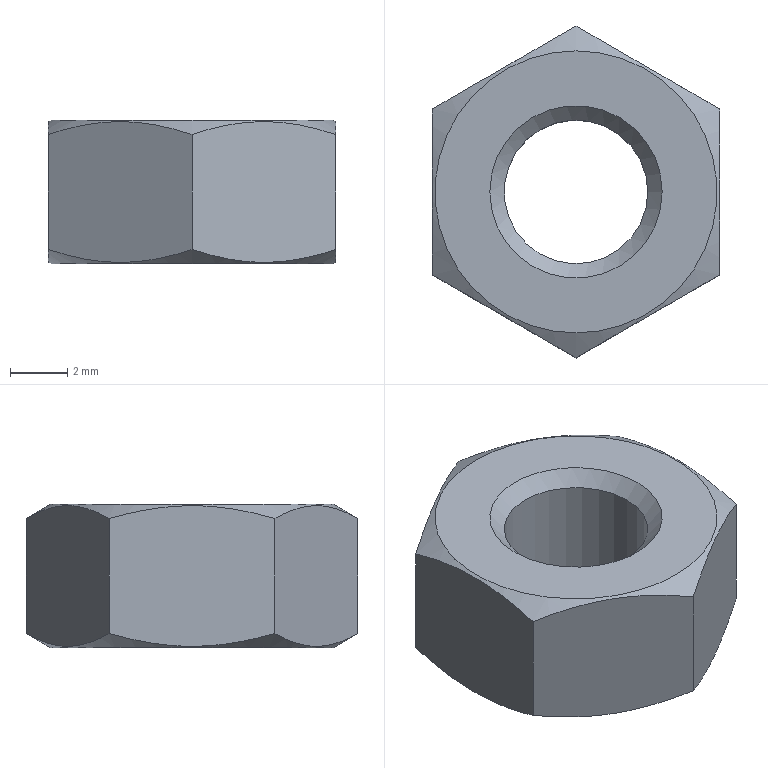Part | NX | features BREP 1, DATUM_CSYS 1 | 1 solid | 13 faces | box 10 x 11.547 x 5 mm | volume 327.462 mm3 | plane 8 | cone 4 | cylinder 1 | commonest cylinder face diameters 5 x1
STEP:
#1=CARTESIAN_POINT('',(-5.,2.887,3.2));
#2=VERTEX_POINT('',#1);
#3=CARTESIAN_POINT('',(-5.,-2.887,3.2));
#4=VERTEX_POINT('',#3);
#5=CARTESIAN_POINT('',(-5.,2.887,3.2));
#6=CARTESIAN_POINT('',(-5.,0.,4.033));
#7=CARTESIAN_POINT('',(-5.,-2.887,3.2));
#8=(BOUNDED_CURVE()B_SPLINE_CURVE(2,(#5,#6,#7),.UNSPECIFIED.,.F.,.F.)B_SPLINE_CURVE_WITH_KNOTS((3,3),(0.,1.),.PIECEWISE_BEZIER_KNOTS.)CURVE()GEOMETRIC_REPRESENTATION_ITEM()RATIONAL_B_SPLINE_CURVE((1.,1.155,1.))REPRESENTATION_ITEM(''));
#9=EDGE_CURVE('',#2,#4,#8,.T.);
#10=ORIENTED_EDGE('',*,*,#9,.F.);
#11=CARTESIAN_POINT('',(-5.,2.887,-0.8));
#12=VERTEX_POINT('',#11);
#13=CARTESIAN_POINT('',(-5.,2.887,3.2));
#14=DIRECTION('',(0.,0.,-1.));
#15=VECTOR('',#14,1000.);
#16=LINE('',#13,#15);
#17=EDGE_CURVE('',#2,#12,#16,.T.);
#18=ORIENTED_EDGE('',*,*,#17,.T.);
#19=CARTESIAN_POINT('',(-5.,-2.887,-0.8));
#20=VERTEX_POINT('',#19);
#21=CARTESIAN_POINT('',(-5.,-2.887,-0.8));
#22=CARTESIAN_POINT('',(-5.,0.,-1.633));
#23=CARTESIAN_POINT('',(-5.,2.887,-0.8));
#24=(BOUNDED_CURVE()B_SPLINE_CURVE(2,(#21,#22,#23),.UNSPECIFIED.,.F.,.F.)B_SPLINE_CURVE_WITH_KNOTS((3,3),(0.,1.),.PIECEWISE_BEZIER_KNOTS.)CURVE()GEOMETRIC_REPRESENTATION_ITEM()RATIONAL_B_SPLINE_CURVE((1.,1.155,1.))REPRESENTATION_ITEM(''));
#25=EDGE_CURVE('',#20,#12,#24,.T.);
#26=ORIENTED_EDGE('',*,*,#25,.F.);
#27=CARTESIAN_POINT('',(-5.,-2.887,3.2));
#28=DIRECTION('',(0.,0.,-1.));
#29=VECTOR('',#28,1000.);
#30=LINE('',#27,#29);
#31=EDGE_CURVE('',#4,#20,#30,.T.);
#32=ORIENTED_EDGE('',*,*,#31,.F.);
#33=EDGE_LOOP('',(#10,#18,#26,#32));
#34=FACE_BOUND('',#33,.T.);
#35=CARTESIAN_POINT('',(-5.,0.,1.2));
#36=DIRECTION('',(1.,0.,0.));
#37=DIRECTION('',(0.,1.,0.));
#38=AXIS2_PLACEMENT_3D('',#35,#36,#37);
#39=PLANE('',#38);
#40=ADVANCED_FACE('',(#34),#39,.F.);
#41=CARTESIAN_POINT('',(0.,-5.774,3.2));
#42=VERTEX_POINT('',#41);
#43=CARTESIAN_POINT('',(-5.,-2.887,3.2));
#44=CARTESIAN_POINT('',(-2.5,-4.33,4.033));
#45=CARTESIAN_POINT('',(0.,-5.774,3.2));
#46=(BOUNDED_CURVE()B_SPLINE_CURVE(2,(#43,#44,#45),.UNSPECIFIED.,.F.,.F.)B_SPLINE_CURVE_WITH_KNOTS((3,3),(0.,1.),.PIECEWISE_BEZIER_KNOTS.)CURVE()GEOMETRIC_REPRESENTATION_ITEM()RATIONAL_B_SPLINE_CURVE((1.,1.155,1.))REPRESENTATION_ITEM(''));
#47=EDGE_CURVE('',#4,#42,#46,.T.);
#48=ORIENTED_EDGE('',*,*,#47,.F.);
#49=ORIENTED_EDGE('',*,*,#31,.T.);
#50=CARTESIAN_POINT('',(0.,-5.774,-0.8));
#51=VERTEX_POINT('',#50);
#52=CARTESIAN_POINT('',(0.,-5.774,-0.8));
#53=CARTESIAN_POINT('',(-2.5,-4.33,-1.633));
#54=CARTESIAN_POINT('',(-5.,-2.887,-0.8));
#55=(BOUNDED_CURVE()B_SPLINE_CURVE(2,(#52,#53,#54),.UNSPECIFIED.,.F.,.F.)B_SPLINE_CURVE_WITH_KNOTS((3,3),(0.,1.),.PIECEWISE_BEZIER_KNOTS.)CURVE()GEOMETRIC_REPRESENTATION_ITEM()RATIONAL_B_SPLINE_CURVE((1.,1.155,1.))REPRESENTATION_ITEM(''));
#56=EDGE_CURVE('',#51,#20,#55,.T.);
#57=ORIENTED_EDGE('',*,*,#56,.F.);
#58=CARTESIAN_POINT('',(0.,-5.774,3.2));
#59=DIRECTION('',(0.,0.,-1.));
#60=VECTOR('',#59,1000.);
#61=LINE('',#58,#60);
#62=EDGE_CURVE('',#42,#51,#61,.T.);
#63=ORIENTED_EDGE('',*,*,#62,.F.);
#64=EDGE_LOOP('',(#48,#49,#57,#63));
#65=FACE_BOUND('',#64,.T.);
#66=CARTESIAN_POINT('',(-2.5,-4.33,1.2));
#67=DIRECTION('',(0.5,0.866,0.));
#68=DIRECTION('',(-0.866,0.5,0.));
#69=AXIS2_PLACEMENT_3D('',#66,#67,#68);
#70=PLANE('',#69);
#71=ADVANCED_FACE('',(#65),#70,.F.);
#72=CARTESIAN_POINT('',(5.,-2.887,3.2));
#73=VERTEX_POINT('',#72);
#74=CARTESIAN_POINT('',(0.,-5.774,3.2));
#75=CARTESIAN_POINT('',(2.5,-4.33,4.033));
#76=CARTESIAN_POINT('',(5.,-2.887,3.2));
#77=(BOUNDED_CURVE()B_SPLINE_CURVE(2,(#74,#75,#76),.UNSPECIFIED.,.F.,.F.)B_SPLINE_CURVE_WITH_KNOTS((3,3),(0.,1.),.PIECEWISE_BEZIER_KNOTS.)CURVE()GEOMETRIC_REPRESENTATION_ITEM()RATIONAL_B_SPLINE_CURVE((1.,1.155,1.))REPRESENTATION_ITEM(''));
#78=EDGE_CURVE('',#42,#73,#77,.T.);
#79=ORIENTED_EDGE('',*,*,#78,.F.);
#80=ORIENTED_EDGE('',*,*,#62,.T.);
#81=CARTESIAN_POINT('',(5.,-2.887,-0.8));
#82=VERTEX_POINT('',#81);
#83=CARTESIAN_POINT('',(5.,-2.887,-0.8));
#84=CARTESIAN_POINT('',(2.5,-4.33,-1.633));
#85=CARTESIAN_POINT('',(0.,-5.774,-0.8));
#86=(BOUNDED_CURVE()B_SPLINE_CURVE(2,(#83,#84,#85),.UNSPECIFIED.,.F.,.F.)B_SPLINE_CURVE_WITH_KNOTS((3,3),(0.,1.),.PIECEWISE_BEZIER_KNOTS.)CURVE()GEOMETRIC_REPRESENTATION_ITEM()RATIONAL_B_SPLINE_CURVE((1.,1.155,1.))REPRESENTATION_ITEM(''));
#87=EDGE_CURVE('',#82,#51,#86,.T.);
#88=ORIENTED_EDGE('',*,*,#87,.F.);
#89=CARTESIAN_POINT('',(5.,-2.887,3.2));
#90=DIRECTION('',(0.,0.,-1.));
#91=VECTOR('',#90,1000.);
#92=LINE('',#89,#91);
#93=EDGE_CURVE('',#73,#82,#92,.T.);
#94=ORIENTED_EDGE('',*,*,#93,.F.);
#95=EDGE_LOOP('',(#79,#80,#88,#94));
#96=FACE_BOUND('',#95,.T.);
#97=CARTESIAN_POINT('',(2.5,-4.33,1.2));
#98=DIRECTION('',(-0.5,0.866,0.));
#99=DIRECTION('',(-0.866,-0.5,0.));
#100=AXIS2_PLACEMENT_3D('',#97,#98,#99);
#101=PLANE('',#100);
#102=ADVANCED_FACE('',(#96),#101,.F.);
#103=CARTESIAN_POINT('',(5.,2.887,3.2));
#104=VERTEX_POINT('',#103);
#105=CARTESIAN_POINT('',(5.,-2.887,3.2));
#106=CARTESIAN_POINT('',(5.,0.,4.033));
#107=CARTESIAN_POINT('',(5.,2.887,3.2));
#108=(BOUNDED_CURVE()B_SPLINE_CURVE(2,(#105,#106,#107),.UNSPECIFIED.,.F.,.F.)B_SPLINE_CURVE_WITH_KNOTS((3,3),(0.,1.),.PIECEWISE_BEZIER_KNOTS.)CURVE()GEOMETRIC_REPRESENTATION_ITEM()RATIONAL_B_SPLINE_CURVE((1.,1.155,1.))REPRESENTATION_ITEM(''));
#109=EDGE_CURVE('',#73,#104,#108,.T.);
#110=ORIENTED_EDGE('',*,*,#109,.F.);
#111=ORIENTED_EDGE('',*,*,#93,.T.);
#112=CARTESIAN_POINT('',(5.,2.887,-0.8));
#113=VERTEX_POINT('',#112);
#114=CARTESIAN_POINT('',(5.,2.887,-0.8));
#115=CARTESIAN_POINT('',(5.,0.,-1.633));
#116=CARTESIAN_POINT('',(5.,-2.887,-0.8));
#117=(BOUNDED_CURVE()B_SPLINE_CURVE(2,(#114,#115,#116),.UNSPECIFIED.,.F.,.F.)B_SPLINE_CURVE_WITH_KNOTS((3,3),(0.,1.),.PIECEWISE_BEZIER_KNOTS.)CURVE()GEOMETRIC_REPRESENTATION_ITEM()RATIONAL_B_SPLINE_CURVE((1.,1.155,1.))REPRESENTATION_ITEM(''));
#118=EDGE_CURVE('',#113,#82,#117,.T.);
#119=ORIENTED_EDGE('',*,*,#118,.F.);
#120=CARTESIAN_POINT('',(5.,2.887,3.2));
#121=DIRECTION('',(0.,0.,-1.));
#122=VECTOR('',#121,1000.);
#123=LINE('',#120,#122);
#124=EDGE_CURVE('',#104,#113,#123,.T.);
#125=ORIENTED_EDGE('',*,*,#124,.F.);
#126=EDGE_LOOP('',(#110,#111,#119,#125));
#127=FACE_BOUND('',#126,.T.);
#128=CARTESIAN_POINT('',(5.,0.,1.2));
#129=DIRECTION('',(-1.,0.,0.));
#130=DIRECTION('',(0.,-1.,0.));
#131=AXIS2_PLACEMENT_3D('',#128,#129,#130);
#132=PLANE('',#131);
#133=ADVANCED_FACE('',(#127),#132,.F.);
#134=CARTESIAN_POINT('',(0.,5.774,3.2));
#135=VERTEX_POINT('',#134);
#136=CARTESIAN_POINT('',(5.,2.887,3.2));
#137=CARTESIAN_POINT('',(2.5,4.33,4.033));
#138=CARTESIAN_POINT('',(0.,5.774,3.2));
#139=(BOUNDED_CURVE()B_SPLINE_CURVE(2,(#136,#137,#138),.UNSPECIFIED.,.F.,.F.)B_SPLINE_CURVE_WITH_KNOTS((3,3),(0.,1.),.PIECEWISE_BEZIER_KNOTS.)CURVE()GEOMETRIC_REPRESENTATION_ITEM()RATIONAL_B_SPLINE_CURVE((1.,1.155,1.))REPRESENTATION_ITEM(''));
#140=EDGE_CURVE('',#104,#135,#139,.T.);
#141=ORIENTED_EDGE('',*,*,#140,.F.);
#142=ORIENTED_EDGE('',*,*,#124,.T.);
#143=CARTESIAN_POINT('',(0.,5.774,-0.8));
#144=VERTEX_POINT('',#143);
#145=CARTESIAN_POINT('',(0.,5.774,-0.8));
#146=CARTESIAN_POINT('',(2.5,4.33,-1.633));
#147=CARTESIAN_POINT('',(5.,2.887,-0.8));
#148=(BOUNDED_CURVE()B_SPLINE_CURVE(2,(#145,#146,#147),.UNSPECIFIED.,.F.,.F.)B_SPLINE_CURVE_WITH_KNOTS((3,3),(0.,1.),.PIECEWISE_BEZIER_KNOTS.)CURVE()GEOMETRIC_REPRESENTATION_ITEM()RATIONAL_B_SPLINE_CURVE((1.,1.155,1.))REPRESENTATION_ITEM(''));
#149=EDGE_CURVE('',#144,#113,#148,.T.);
#150=ORIENTED_EDGE('',*,*,#149,.F.);
#151=CARTESIAN_POINT('',(0.,5.774,3.2));
#152=DIRECTION('',(0.,0.,-1.));
#153=VECTOR('',#152,1000.);
#154=LINE('',#151,#153);
#155=EDGE_CURVE('',#135,#144,#154,.T.);
#156=ORIENTED_EDGE('',*,*,#155,.F.);
#157=EDGE_LOOP('',(#141,#142,#150,#156));
#158=FACE_BOUND('',#157,.T.);
#159=CARTESIAN_POINT('',(2.5,4.33,1.2));
#160=DIRECTION('',(-0.5,-0.866,0.));
#161=DIRECTION('',(0.866,-0.5,0.));
#162=AXIS2_PLACEMENT_3D('',#159,#160,#161);
#163=PLANE('',#162);
#164=ADVANCED_FACE('',(#158),#163,.F.);
#165=CARTESIAN_POINT('',(0.,5.774,3.2));
#166=CARTESIAN_POINT('',(-2.5,4.33,4.033));
#167=CARTESIAN_POINT('',(-5.,2.887,3.2));
#168=(BOUNDED_CURVE()B_SPLINE_CURVE(2,(#165,#166,#167),.UNSPECIFIED.,.F.,.F.)B_SPLINE_CURVE_WITH_KNOTS((3,3),(0.,1.),.PIECEWISE_BEZIER_KNOTS.)CURVE()GEOMETRIC_REPRESENTATION_ITEM()RATIONAL_B_SPLINE_CURVE((1.,1.155,1.))REPRESENTATION_ITEM(''));
#169=EDGE_CURVE('',#135,#2,#168,.T.);
#170=ORIENTED_EDGE('',*,*,#169,.F.);
#171=ORIENTED_EDGE('',*,*,#155,.T.);
#172=CARTESIAN_POINT('',(-5.,2.887,-0.8));
#173=CARTESIAN_POINT('',(-2.5,4.33,-1.633));
#174=CARTESIAN_POINT('',(0.,5.774,-0.8));
#175=(BOUNDED_CURVE()B_SPLINE_CURVE(2,(#172,#173,#174),.UNSPECIFIED.,.F.,.F.)B_SPLINE_CURVE_WITH_KNOTS((3,3),(0.,1.),.PIECEWISE_BEZIER_KNOTS.)CURVE()GEOMETRIC_REPRESENTATION_ITEM()RATIONAL_B_SPLINE_CURVE((1.,1.155,1.))REPRESENTATION_ITEM(''));
#176=EDGE_CURVE('',#12,#144,#175,.T.);
#177=ORIENTED_EDGE('',*,*,#176,.F.);
#178=ORIENTED_EDGE('',*,*,#17,.F.);
#179=EDGE_LOOP('',(#170,#171,#177,#178));
#180=FACE_BOUND('',#179,.T.);
#181=CARTESIAN_POINT('',(-2.5,4.33,1.2));
#182=DIRECTION('',(0.5,-0.866,0.));
#183=DIRECTION('',(0.866,0.5,0.));
#184=AXIS2_PLACEMENT_3D('',#181,#182,#183);
#185=PLANE('',#184);
#186=ADVANCED_FACE('',(#180),#185,.F.);
#187=CARTESIAN_POINT('',(0.,4.907,3.7));
#188=VERTEX_POINT('',#187);
#189=CARTESIAN_POINT('',(0.,0.,3.7));
#190=DIRECTION('',(0.,0.,1.));
#191=DIRECTION('',(0.,1.,0.));
#192=AXIS2_PLACEMENT_3D('',#189,#190,#191);
#193=CIRCLE('',#192,4.907);
#194=EDGE_CURVE('',#188,#188,#193,.T.);
#195=ORIENTED_EDGE('',*,*,#194,.T.);
#196=EDGE_LOOP('',(#195));
#197=FACE_BOUND('',#196,.T.);
#198=CARTESIAN_POINT('',(3.,0.,3.7));
#199=VERTEX_POINT('',#198);
#200=CARTESIAN_POINT('',(0.,0.,3.7));
#201=DIRECTION('',(0.,0.,1.));
#202=DIRECTION('',(1.,0.,0.));
#203=AXIS2_PLACEMENT_3D('',#200,#201,#202);
#204=CIRCLE('',#203,3.);
#205=EDGE_CURVE('',#199,#199,#204,.T.);
#206=ORIENTED_EDGE('',*,*,#205,.F.);
#207=EDGE_LOOP('',(#206));
#208=FACE_BOUND('',#207,.T.);
#209=CARTESIAN_POINT('',(-0.2194,-0.6375,3.7));
#210=DIRECTION('',(0.,0.,1.));
#211=DIRECTION('',(-1.,0.,0.));
#212=AXIS2_PLACEMENT_3D('',#209,#210,#211);
#213=PLANE('',#212);
#214=ADVANCED_FACE('',(#197,#208),#213,.T.);
#215=CARTESIAN_POINT('',(0.,4.907,-1.3));
#216=VERTEX_POINT('',#215);
#217=CARTESIAN_POINT('',(0.,0.,-1.3));
#218=DIRECTION('',(0.,0.,1.));
#219=DIRECTION('',(0.,1.,0.));
#220=AXIS2_PLACEMENT_3D('',#217,#218,#219);
#221=CIRCLE('',#220,4.907);
#222=EDGE_CURVE('',#216,#216,#221,.T.);
#223=ORIENTED_EDGE('',*,*,#222,.F.);
#224=EDGE_LOOP('',(#223));
#225=FACE_BOUND('',#224,.T.);
#226=CARTESIAN_POINT('',(3.,0.,-1.3));
#227=VERTEX_POINT('',#226);
#228=CARTESIAN_POINT('',(0.,0.,-1.3));
#229=DIRECTION('',(0.,0.,1.));
#230=DIRECTION('',(1.,0.,0.));
#231=AXIS2_PLACEMENT_3D('',#228,#229,#230);
#232=CIRCLE('',#231,3.);
#233=EDGE_CURVE('',#227,#227,#232,.T.);
#234=ORIENTED_EDGE('',*,*,#233,.T.);
#235=EDGE_LOOP('',(#234));
#236=FACE_BOUND('',#235,.T.);
#237=CARTESIAN_POINT('',(-0.2194,-0.6375,-1.3));
#238=DIRECTION('',(0.,0.,1.));
#239=DIRECTION('',(-1.,0.,0.));
#240=AXIS2_PLACEMENT_3D('',#237,#238,#239);
#241=PLANE('',#240);
#242=ADVANCED_FACE('',(#225,#236),#241,.F.);
#243=CARTESIAN_POINT('',(2.5,0.,3.2));
#244=VERTEX_POINT('',#243);
#245=CARTESIAN_POINT('',(2.5,0.,-0.8));
#246=VERTEX_POINT('',#245);
#247=CARTESIAN_POINT('',(2.5,0.,3.2));
#248=DIRECTION('',(0.,0.,-1.));
#249=VECTOR('',#248,1000.);
#250=LINE('',#247,#249);
#251=EDGE_CURVE('',#244,#246,#250,.T.);
#252=ORIENTED_EDGE('',*,*,#251,.T.);
#253=CARTESIAN_POINT('',(0.,0.,-0.8));
#254=DIRECTION('',(0.,0.,1.));
#255=DIRECTION('',(1.,0.,0.));
#256=AXIS2_PLACEMENT_3D('',#253,#254,#255);
#257=CIRCLE('',#256,2.5);
#258=EDGE_CURVE('',#246,#246,#257,.T.);
#259=ORIENTED_EDGE('',*,*,#258,.F.);
#260=ORIENTED_EDGE('',*,*,#251,.F.);
#261=CARTESIAN_POINT('',(0.,0.,3.2));
#262=DIRECTION('',(0.,0.,1.));
#263=DIRECTION('',(1.,0.,0.));
#264=AXIS2_PLACEMENT_3D('',#261,#262,#263);
#265=CIRCLE('',#264,2.5);
#266=EDGE_CURVE('',#244,#244,#265,.T.);
#267=ORIENTED_EDGE('',*,*,#266,.T.);
#268=EDGE_LOOP('',(#252,#259,#260,#267));
#269=FACE_BOUND('',#268,.T.);
#270=CARTESIAN_POINT('',(0.,0.,3.7));
#271=DIRECTION('',(0.,0.,-1.));
#272=DIRECTION('',(-1.,0.,0.));
#273=AXIS2_PLACEMENT_3D('',#270,#271,#272);
#274=CYLINDRICAL_SURFACE('',#273,2.5);
#275=ADVANCED_FACE('',(#269),#274,.F.);
#276=CARTESIAN_POINT('',(2.5,0.,3.2));
#277=DIRECTION('',(0.7071,0.,0.7071));
#278=VECTOR('',#277,1000.);
#279=LINE('',#276,#278);
#280=EDGE_CURVE('',#244,#199,#279,.T.);
#281=ORIENTED_EDGE('',*,*,#280,.F.);
#282=ORIENTED_EDGE('',*,*,#266,.F.);
#283=ORIENTED_EDGE('',*,*,#280,.T.);
#284=ORIENTED_EDGE('',*,*,#205,.T.);
#285=EDGE_LOOP('',(#281,#282,#283,#284));
#286=FACE_BOUND('',#285,.T.);
#287=CARTESIAN_POINT('',(0.,0.,3.2));
#288=DIRECTION('',(0.,0.,1.));
#289=DIRECTION('',(-1.,0.,0.));
#290=AXIS2_PLACEMENT_3D('',#287,#288,#289);
#291=CONICAL_SURFACE('',#290,2.5,0.7854);
#292=ADVANCED_FACE('',(#286),#291,.F.);
#293=ORIENTED_EDGE('',*,*,#233,.F.);
#294=CARTESIAN_POINT('',(3.,0.,-1.3));
#295=DIRECTION('',(-0.7071,0.,0.7071));
#296=VECTOR('',#295,1000.);
#297=LINE('',#294,#296);
#298=EDGE_CURVE('',#227,#246,#297,.T.);
#299=ORIENTED_EDGE('',*,*,#298,.T.);
#300=ORIENTED_EDGE('',*,*,#258,.T.);
#301=ORIENTED_EDGE('',*,*,#298,.F.);
#302=EDGE_LOOP('',(#293,#299,#300,#301));
#303=FACE_BOUND('',#302,.T.);
#304=CARTESIAN_POINT('',(0.,0.,-0.8));
#305=DIRECTION('',(0.,0.,-1.));
#306=DIRECTION('',(-1.,0.,0.));
#307=AXIS2_PLACEMENT_3D('',#304,#305,#306);
#308=CONICAL_SURFACE('',#307,2.5,0.7854);
#309=ADVANCED_FACE('',(#303),#308,.F.);
#310=CARTESIAN_POINT('',(0.,5.774,-0.8));
#311=DIRECTION('',(0.,-0.866,-0.5));
#312=VECTOR('',#311,1000.);
#313=LINE('',#310,#312);
#314=EDGE_CURVE('',#144,#216,#313,.T.);
#315=ORIENTED_EDGE('',*,*,#314,.T.);
#316=ORIENTED_EDGE('',*,*,#222,.T.);
#317=ORIENTED_EDGE('',*,*,#314,.F.);
#318=ORIENTED_EDGE('',*,*,#149,.T.);
#319=ORIENTED_EDGE('',*,*,#118,.T.);
#320=ORIENTED_EDGE('',*,*,#87,.T.);
#321=ORIENTED_EDGE('',*,*,#56,.T.);
#322=ORIENTED_EDGE('',*,*,#25,.T.);
#323=ORIENTED_EDGE('',*,*,#176,.T.);
#324=EDGE_LOOP('',(#315,#316,#317,#318,#319,#320,#321,#322,#323));
#325=FACE_BOUND('',#324,.T.);
#326=CARTESIAN_POINT('',(0.,0.,-1.3));
#327=DIRECTION('',(0.,0.,1.));
#328=DIRECTION('',(0.,-1.,0.));
#329=AXIS2_PLACEMENT_3D('',#326,#327,#328);
#330=CONICAL_SURFACE('',#329,4.907,1.047);
#331=ADVANCED_FACE('',(#325),#330,.T.);
#332=CARTESIAN_POINT('',(0.,4.907,3.7));
#333=DIRECTION('',(0.,0.866,-0.5));
#334=VECTOR('',#333,1000.);
#335=LINE('',#332,#334);
#336=EDGE_CURVE('',#188,#135,#335,.T.);
#337=ORIENTED_EDGE('',*,*,#336,.T.);
#338=ORIENTED_EDGE('',*,*,#169,.T.);
#339=ORIENTED_EDGE('',*,*,#9,.T.);
#340=ORIENTED_EDGE('',*,*,#47,.T.);
#341=ORIENTED_EDGE('',*,*,#78,.T.);
#342=ORIENTED_EDGE('',*,*,#109,.T.);
#343=ORIENTED_EDGE('',*,*,#140,.T.);
#344=ORIENTED_EDGE('',*,*,#336,.F.);
#345=ORIENTED_EDGE('',*,*,#194,.F.);
#346=EDGE_LOOP('',(#337,#338,#339,#340,#341,#342,#343,#344,#345));
#347=FACE_BOUND('',#346,.T.);
#348=CARTESIAN_POINT('',(0.,0.,3.7));
#349=DIRECTION('',(0.,0.,-1.));
#350=DIRECTION('',(0.,-1.,0.));
#351=AXIS2_PLACEMENT_3D('',#348,#349,#350);
#352=CONICAL_SURFACE('',#351,4.907,1.047);
#353=ADVANCED_FACE('',(#347),#352,.T.);
#354=CLOSED_SHELL('',(#40,#71,#102,#133,#164,#186,#214,#242,#275,#292,#309,#331,#353));
#355=MANIFOLD_SOLID_BREP('',#354);
#356=(LENGTH_UNIT()NAMED_UNIT(*)SI_UNIT(.MILLI.,.METRE.));
#357=UNCERTAINTY_MEASURE_WITH_UNIT(LENGTH_MEASURE(0.00001),#356,'','');
#358=(NAMED_UNIT(*)PLANE_ANGLE_UNIT()SI_UNIT($,.RADIAN.));
#359=(NAMED_UNIT(*)SI_UNIT($,.STERADIAN.)SOLID_ANGLE_UNIT());
#360=(GEOMETRIC_REPRESENTATION_CONTEXT(3)GLOBAL_UNCERTAINTY_ASSIGNED_CONTEXT((#357))GLOBAL_UNIT_ASSIGNED_CONTEXT((#356,#358,#359))REPRESENTATION_CONTEXT('',''));
#361=ADVANCED_BREP_SHAPE_REPRESENTATION('',(#355),#360);